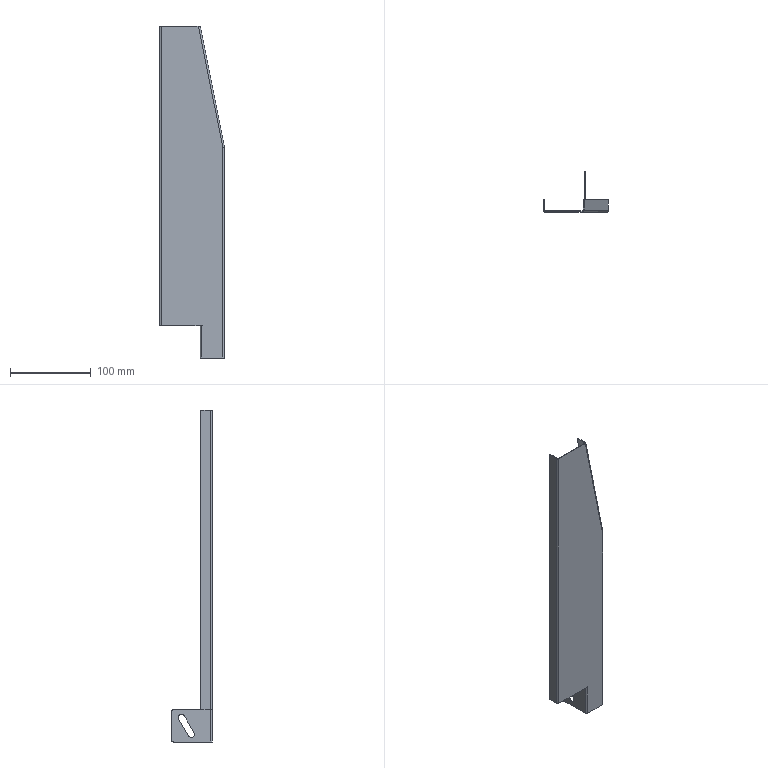Part | 1 solid | 58 faces | box 80 x 50 x 410 mm | volume 48681 mm3 | plane 39 | cylinder 17 | spline 2 | commonest cylinder face diameters 4 x6 1.473 x4 3.873 x4 8 x3